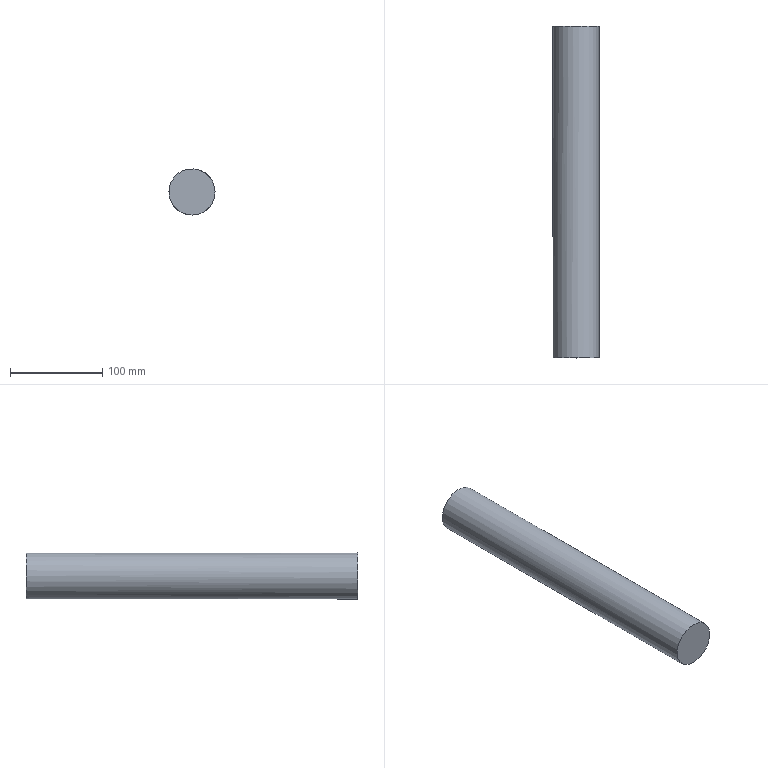Part | NX | features solid 2 | 1 solid | 3 faces | box 50 x 360 x 50 mm | volume 706858 mm3 | plane 2 | cylinder 1 | commonest cylinder face diameters 50 x1
STEP:
#1=CARTESIAN_POINT('',(142.,-535.,-235.5));
#2=VERTEX_POINT('',#1);
#3=CARTESIAN_POINT('',(142.,-535.,-210.5));
#4=DIRECTION('',(0.,-1.,0.));
#5=DIRECTION('',(0.,0.,-1.));
#6=AXIS2_PLACEMENT_3D('',#3,#4,#5);
#7=CIRCLE('',#6,25.);
#8=EDGE_CURVE('',#2,#2,#7,.F.);
#9=ORIENTED_EDGE('',*,*,#8,.F.);
#10=EDGE_LOOP('',(#9));
#11=FACE_BOUND('',#10,.T.);
#12=CARTESIAN_POINT('',(142.,-535.,-210.5));
#13=DIRECTION('',(0.,-1.,0.));
#14=DIRECTION('',(0.,0.,-1.));
#15=AXIS2_PLACEMENT_3D('',#12,#13,#14);
#16=PLANE('',#15);
#17=ADVANCED_FACE('',(#11),#16,.T.);
#18=CARTESIAN_POINT('',(167.,-175.,-210.5));
#19=VERTEX_POINT('',#18);
#20=CARTESIAN_POINT('',(142.,-175.,-210.5));
#21=DIRECTION('',(0.,-1.,0.));
#22=DIRECTION('',(1.,0.,0.));
#23=AXIS2_PLACEMENT_3D('',#20,#21,#22);
#24=CIRCLE('',#23,25.);
#25=EDGE_CURVE('',#19,#19,#24,.T.);
#26=ORIENTED_EDGE('',*,*,#25,.F.);
#27=EDGE_LOOP('',(#26));
#28=FACE_BOUND('',#27,.T.);
#29=CARTESIAN_POINT('',(142.,-175.,-210.5));
#30=DIRECTION('',(0.,1.,0.));
#31=DIRECTION('',(0.,0.,1.));
#32=AXIS2_PLACEMENT_3D('',#29,#30,#31);
#33=PLANE('',#32);
#34=ADVANCED_FACE('',(#28),#33,.T.);
#35=ORIENTED_EDGE('',*,*,#8,.T.);
#36=EDGE_LOOP('',(#35));
#37=FACE_BOUND('',#36,.T.);
#38=ORIENTED_EDGE('',*,*,#25,.T.);
#39=EDGE_LOOP('',(#38));
#40=FACE_BOUND('',#39,.T.);
#41=CARTESIAN_POINT('',(142.,-175.,-210.5));
#42=DIRECTION('',(0.,-1.,0.));
#43=DIRECTION('',(1.,0.,0.));
#44=AXIS2_PLACEMENT_3D('',#41,#42,#43);
#45=CYLINDRICAL_SURFACE('',#44,25.);
#46=ADVANCED_FACE('',(#37,#40),#45,.T.);
#47=CLOSED_SHELL('',(#17,#34,#46));
#48=MANIFOLD_SOLID_BREP('',#47);
#49=(LENGTH_UNIT()NAMED_UNIT(*)SI_UNIT(.MILLI.,.METRE.));
#50=UNCERTAINTY_MEASURE_WITH_UNIT(LENGTH_MEASURE(0.00001),#49,'','');
#51=(NAMED_UNIT(*)PLANE_ANGLE_UNIT()SI_UNIT($,.RADIAN.));
#52=(NAMED_UNIT(*)SI_UNIT($,.STERADIAN.)SOLID_ANGLE_UNIT());
#53=(GEOMETRIC_REPRESENTATION_CONTEXT(3)GLOBAL_UNCERTAINTY_ASSIGNED_CONTEXT((#50))GLOBAL_UNIT_ASSIGNED_CONTEXT((#49,#51,#52))REPRESENTATION_CONTEXT('',''));
#54=ADVANCED_BREP_SHAPE_REPRESENTATION('',(#48),#53);